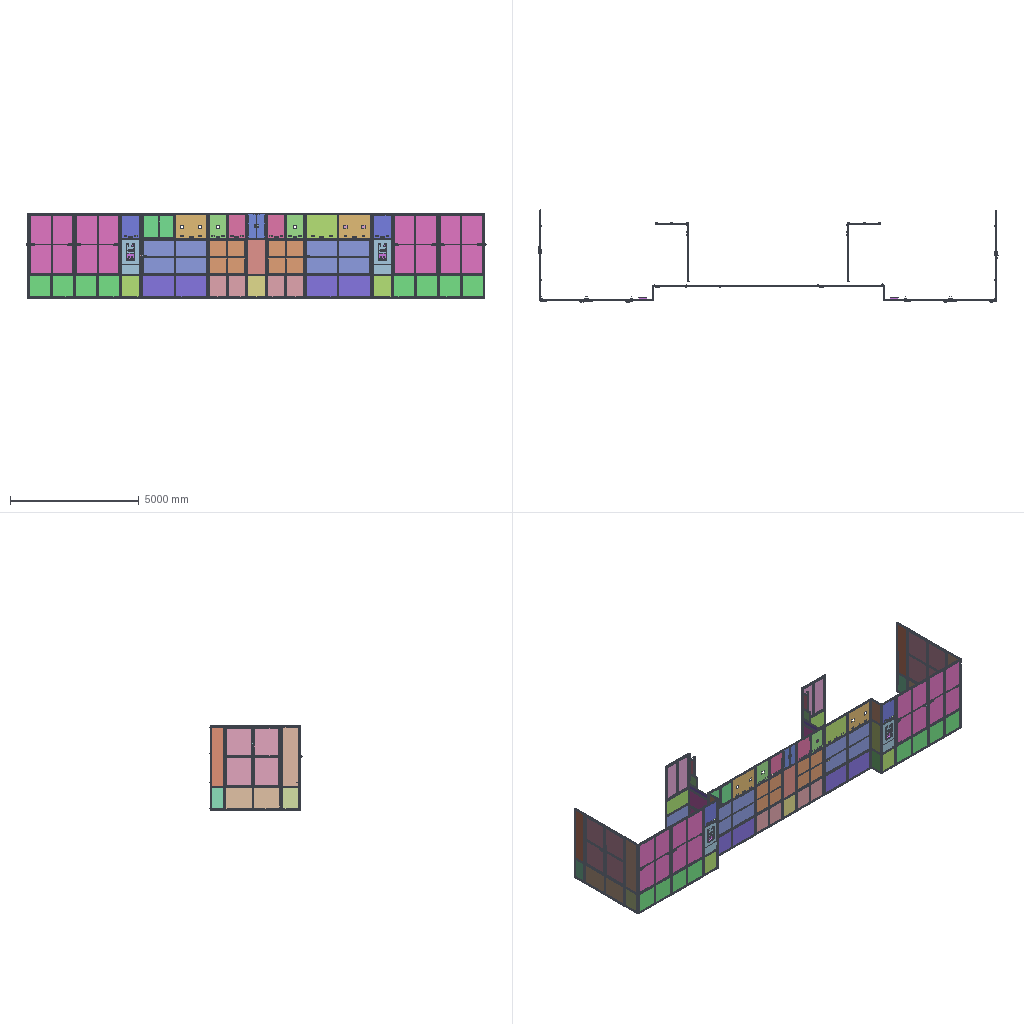Assembly | SolidWorks | 258 different items | 3509 placed | box 17871 x 3575 x 3280 mm
Parts list (item | name | quantity | parent item | size | volume | features):
1 | (subassembly) | x2 | in 6, 44 | - | 15381691 mm3 | features ReferencePattern 29, LocalLPattern 9
2 | (subassembly) | x2 | in 6, 44 | 1336 x 15 x 720 mm | 5449315 mm3 | features ReferencePattern 3, LocalLPattern 2
3 | (subassembly) | x2 | in 6, 44 | 1336 x 15 x 720 mm | 5449313 mm3 | features ReferencePattern 3, LocalLPattern 2
4 | (subassembly) | x2 | in 6, 44 | 685 x 936.5 x 44 mm | 1299683 mm3 | -
5 | (subassembly) | x2 | in 6, 44 | 685 x 936.5 x 44 mm | 1322747 mm3 | -
6 | (subassembly) | x1 | - | - | 28902679 mm3 | -
7 | (subassembly) | x1 | - | - | 60412715 mm3 | -
8 | (subassembly) | x1 | in 7 | - | 23168671 mm3 | features ReferencePattern 57, LocalLPattern 9, CompositeCurve 4, DerivedHolePattern 2
9 | (subassembly) | x1 | in 7 | 1225 x 936.5 x 44 mm | 2159359 mm3 | -
10 | (subassembly) | x1 | - | - | 65477431 mm3 | -
11 | (subassembly) | x1 | - | - | 15444382 mm3 | -
12 | (subassembly) | x1 | in 10 | - | 24079558 mm3 | features ReferencePattern 37, LocalLPattern 9, CompositeCurve 6
13 | (subassembly) | x2 | in 7, 10 | 1336 x 15 x 1260 mm | 9289979 mm3 | features ReferencePattern 3, LocalLPattern 2
14 | (subassembly) | x2 | in 7, 10 | 1336 x 89 x 1260 mm | 9587971 mm3 | features ReferencePattern 3, LocalLPattern 2
15 | (subassembly) | x2 | in 7, 10 | 595.4 x 40 x 3280 mm | 13933282 mm3 | features ReferencePattern 20, LocalLPattern 6
16 | (subassembly) | x1 | in 10 | 902 x 84 x 625 mm | 3238320 mm3 | features ReferencePattern 5, LocalLPattern 1
17 | (subassembly) | x1 | in 10 | 902 x 68 x 625 mm | 3235743 mm3 | features ReferencePattern 5, LocalLPattern 1
18 | (subassembly) | x2 | in 7, 10 | 1225 x 936.5 x 44 mm | 2112957 mm3 | -
19 | (subassembly) | x2 | - | 720.4 x 40 x 3280 mm | 15751167 mm3 | features ReferencePattern 12, LocalLPattern 4
20 | (subassembly) | x2 | - | - | - | -
21 | (subassembly) | x2 | in 20 | - | 17892849 mm3 | features ReferencePattern 36, LocalLPattern 3, DerivedHolePattern 1, MirrorCompFeat 1
22 | (subassembly) | x1 | in 11 | 772.4 x 40 x 3280 mm | 13403212 mm3 | features ReferencePattern 21, LocalLPattern 5, CompositeCurve 2
23 | (subassembly) | x4 | in 20 | - | - | features ReferencePattern 51, LocalLPattern 7, CompositeCurve 4
24 | (subassembly) | x2 | - | 562.4 x 40 x 3280 mm | 12898463 mm3 | features ReferencePattern 12, LocalLPattern 4
25 | (subassembly) | x2 | - | - | 29193097 mm3 | features ReferencePattern 104, MirrorCompFeat 10, LocalLPattern 4, DerivedHolePattern 1
26 | (subassembly) | x2 | - | - | 29490939 mm3 | -
27 | (subassembly) | x2 | in 26 | 40 x 3280 x 1290 mm | 16940253 mm3 | features ReferencePattern 22, LocalLPattern 5, MirrorCompFeat 2, CompositeCurve 1
28 | (subassembly) | x4 | in 26 | 633 x 92.5 x 1575 mm | 6275343 mm3 | features ReferencePattern 36, LocalLPattern 7, CompositeCurve 3
29 | (subassembly) | x4 | - | - | - | features CompositeCurve 1
30 | (subassembly) | x4 | in 29 | - | 16081270 mm3 | features ReferencePattern 57, LocalLPattern 5, CompositeCurve 3
31 | (subassembly) | x4 | in 29 | 2296 x 92.007 x 864.302 mm | 10874128 mm3 | features ReferencePattern 7, LocalLPattern 2
32 | (subassembly) | x4 | in 29 | - | 11302855 mm3 | features ReferencePattern 6, LocalLPattern 3
33 | (subassembly) | x2 | in 11 | 349.5 x 954 x 47.25 mm | 1020587 mm3 | features ReferencePattern 5, LocalLPattern 1
34 | (subassembly) | x526 | in 1, 8, 12, 15, 19, 21, 22, 23, 24, 25, 27, 28, 30, 41 | - | - | -
35 | (subassembly) | x4 | in 33 | 44.75 x 12.6 x 82 mm | 29571 mm3 | -
36 | (subassembly) | x2 | in 21 | - | - | -
37 | (subassembly) | x20 | in 23, 28 | 62 x 12.05 x 82 mm | 23876 mm3 | -
38 | (subassembly) | x16 | in 1, 8, 12, 30 | - | - | -
39 | (subassembly) | x1 | in 7 | - | 117384 mm3 | -
40 | (subassembly) | x2 | - | - | 12397020 mm3 | -
41 | (subassembly) | x2 | in 40 | 792.4 x 40 x 3280 mm | 8824321 mm3 | features ReferencePattern 12, LocalLPattern 3
42 | (subassembly) | x2 | in 40 | 697 x 1379 x 104.25 mm | 2244190 mm3 | features ReferencePattern 6, DerivedHolePattern 1
43 | (subassembly) | x2 | in 40 | 695 x 928.5 x 44 mm | 1328508 mm3 | -
44 | (subassembly) | x1 | - | - | 28902679 mm3 | -
45 | - | x2 | in 18 | 1225 x 925 x 38 mm | 1989320 mm3 | features ICE 7, SMWeldBead 4, EdgeFlange 2, FlatPattern 1, HoleWzd 1, SMBaseFlange 1, SheetMetal 1
46 | - | x8 | in 19, 24 | 14 x 20.3 x 2314 mm | 117819 mm3 | features BaseBody 1, ICE 1, MoveFace 1
47 | - | x4 | in 25 | 14 x 20.3 x 320 mm | 16293 mm3 | features BaseBody 1, ICE 1, MoveFace 1
48 | - | x4 | in 25 | 14 x 20.3 x 420 mm | 21385 mm3 | features BaseBody 1, ICE 1, MoveFace 1
49 | - | x20 | in 15, 24 | 14 x 20.3 x 410 mm | 20875 mm3 | features BaseBody 1, ICE 1, MoveFace 1
50 | - | x8 | in 28 | 14 x 20.3 x 461 mm | 23472 mm3 | features BaseBody 1, ICE 1, MoveFace 1
51 | - | x8 | in 19 | 14 x 20.3 x 568 mm | 28920 mm3 | features BaseBody 1, ICE 1, MoveFace 1
52 | - | x4 | in 41 | 14 x 20.3 x 606 mm | 30855 mm3 | features BaseBody 1, ICE 1, MoveFace 1
53 | - | x4 | in 22 | 14 x 20.3 x 620 mm | 31568 mm3 | features BaseBody 1, ICE 1, MoveFace 1
54 | - | x8 | in 1 | 14 x 20.3 x 657 mm | 33452 mm3 | features BaseBody 1, ICE 1, MoveFace 1
55 | - | x16 | in 25 | 14 x 20.3 x 670 mm | 34114 mm3 | features BaseBody 1, ICE 1, MoveFace 1
56 | - | x4 | in 32 | 23 x 25 x 60 mm | 5085 mm3 | features HoleWzd 2, Chamfer 1, FlatPattern 1, SMBaseFlange 1, SheetMetal 1
57 | - | x4 | in 27 | 14 x 20.3 x 692 mm | 35234 mm3 | features BaseBody 1, ICE 1, MoveFace 1
58 | - | x4 | in 25 | 14 x 20.3 x 730 mm | 37168 mm3 | features BaseBody 1, ICE 1, MoveFace 1
59 | - | x20 | in 1, 8, 12, 21, 30 | 14 x 20.3 x 786 mm | 40020 mm3 | features BaseBody 1, ICE 1, MoveFace 1
60 | - | x20 | in 21, 30 | 14 x 20.3 x 800 mm | 40733 mm3 | features BaseBody 1, ICE 1, MoveFace 1
61 | - | x4 | in 27 | 14 x 20.3 x 842 mm | 42871 mm3 | features BaseBody 1, ICE 1, MoveFace 1
62 | - | x37 | in 1, 8, 12, 15, 19, 22, 24, 30, 41 | 14 x 20.3 x 856 mm | 43584 mm3 | features BaseBody 1, ICE 1, MoveFace 1
63 | - | x4 | in 15 | 14 x 20.3 x 914 mm | 46537 mm3 | features BaseBody 1, ICE 1, MoveFace 1
64 | - | x16 | in 23 | 14 x 20.3 x 915 mm | 46588 mm3 | features BaseBody 1, ICE 1, MoveFace 1
65 | - | x8 | in 13, 14 | 30 x 15 x 1200 mm | 289403 mm3 | features BaseBody 1, MoveFace 1
66 | - | x4 | in 13, 14 | 30 x 15 x 1200 mm | 289001 mm3 | features BaseBody 1, HoleWzd 1, MoveFace 1
67 | - | x10 | in 16, 31 | 39 x 17 x 40 mm | 4045 mm3 | features HoleWzd 2, FlatPattern 1, SMBaseFlange 1, SheetMetal 1
68 | - | x4 | in 13, 14 | 30 x 15 x 1276 mm | 306850 mm3 | features HoleWzd 3, BaseBody 1, MoveFace 1
69 | - | x12 | in 2, 3, 13, 14 | 30 x 15 x 1276 mm | 307460 mm3 | features BaseBody 1, HoleWzd 1, MoveFace 1
70 | - | x8 | in 31, 32 | 30 x 15 x 2236 mm | 538276 mm3 | features HoleWzd 3, BaseBody 1, MoveFace 1
71 | - | x8 | in 31, 32 | 30 x 15 x 2236 mm | 538982 mm3 | features BaseBody 1, HoleWzd 1, MoveFace 1
72 | - | x4 | in 16, 17 | 30 x 15 x 565 mm | 136260 mm3 | features BaseBody 1, MoveFace 1
73 | - | x8 | in 2, 3 | 30 x 15 x 660 mm | 159171 mm3 | features BaseBody 1, MoveFace 1
74 | - | x4 | in 2, 3 | 30 x 15 x 660 mm | 158770 mm3 | features BaseBody 1, HoleWzd 1, MoveFace 1
75 | - | x20 | in 31, 32 | 30 x 15 x 802 mm | 193417 mm3 | features BaseBody 1, MoveFace 1
76 | - | x4 | in 32 | 30 x 15 x 802 mm | 193016 mm3 | features BaseBody 1, HoleWzd 1, MoveFace 1
77 | - | x2 | in 16, 17 | 30 x 15 x 842 mm | 202454 mm3 | features HoleWzd 2, BaseBody 1, MoveFace 1
78 | - | x18 | in 8, 30 | 17.5 x 17 x 60 mm | 3562 mm3 | features HoleWzd 2, FlatPattern 1, SMBaseFlange 1, SheetMetal 1
79 | - | x2 | in 16, 17 | 30 x 15 x 842 mm | 203064 mm3 | features BaseBody 1, MoveFace 1
80 | - | x2 | in 25 | 40 x 40 x 1548 mm | 930498 mm3 | features Extrusion 1
81 | - | x8 | in 25 | 40 x 40 x 2144 mm | 1280370 mm3 | features Extrusion 1, HoleWzd 1
82 | - | x2 | in 25 | 40 x 40 x 240 mm | 135882 mm3 | features Extrusion 1, HoleWzd 1
83 | - | x2 | in 25 | 40 x 40 x 2470 mm | 1483507 mm3 | features HoleWzd 2, Extrusion 1
84 | - | x4 | in 25 | 40 x 40 x 400 mm | 232057 mm3 | features Extrusion 1, HoleWzd 1
85 | - | x2 | in 25 | 40 x 40 x 410 mm | 238068 mm3 | features Extrusion 1, HoleWzd 1
86 | - | x2 | in 25 | 40 x 40 x 454 mm | 264516 mm3 | features Extrusion 1, HoleWzd 1
87 | - | x4 | in 25 | 40 x 40 x 730 mm | 430419 mm3 | features Extrusion 1, HoleWzd 1
88 | - | x4 | in 25 | 40 x 40 x 810 mm | 486492 mm3 | features HoleWzd 2, Extrusion 1
89 | - | x10 | in 17, 32 | 23 x 17 x 40 mm | 2765 mm3 | features HoleWzd 2, FlatPattern 1, SMBaseFlange 1, SheetMetal 1
90 | - | x2 | in 25 | 40 x 40 x 922 mm | 554211 mm3 | features Extrusion 1
91 | - | x8 | in 27 | 40 x 40 x 1210 mm | 708024 mm3 | features BaseBody 1, HoleWzd 1, MoveFace 1
92 | - | x8 | in 1 | 40 x 40 x 1420 mm | 832360 mm3 | features BaseBody 1, HoleWzd 1, MoveFace 1
93 | - | x12 | in 30 | 40 x 40 x 1705 mm | 1001101 mm3 | features BaseBody 1, HoleWzd 1, MoveFace 1
94 | - | x6 | in 21 | 40 x 40 x 2120 mm | 1246811 mm3 | features BaseBody 1, HoleWzd 1, MoveFace 1
95 | - | x8 | in 8, 12 | 40 x 40 x 2500 mm | 1471799 mm3 | features BaseBody 1, HoleWzd 1, MoveFace 1
96 | - | x3 | in 1, 12 | 40 x 40 x 3280 mm | 1938828 mm3 | features HoleWzd 5, BaseBody 1, MoveFace 1
97 | - | x3 | in 1, 12 | 40 x 40 x 3280 mm | 1938828 mm3 | features HoleWzd 5, BaseBody 1, MoveFace 1
98 | - | x4 | in 21 | 40 x 40 x 3280 mm | 1937764 mm3 | features HoleWzd 4, BaseBody 1, MoveFace 1
99 | - | x8 | in 19, 24 | 40 x 40 x 3280 mm | 1939169 mm3 | features HoleWzd 4, 3DProfileFeature 1, BaseBody 1, MoveFace 1
100 | - | x12 | in 21 | 72 x 17 x 32 mm | 6272 mm3 | features Chamfer 1, FlatPattern 1, HoleWzd 1, SMBaseFlange 1, SheetMetal 1
101 | - | x4 | in 27 | 40 x 40 x 3280 mm | 1937764 mm3 | features HoleWzd 4, BaseBody 1, MoveFace 1
102 | - | x16 | in 8, 15, 22, 30, 41 | 40 x 40 x 3280 mm | 1939654 mm3 | features HoleWzd 3, BaseBody 1, MoveFace 1
103 | - | x4 | in 30 | 40 x 40 x 3280 mm | 1938824 mm3 | features HoleWzd 5, BaseBody 1, MoveFace 1
104 | - | x6 | in 24 | 40 x 40 x 470 mm | 269890 mm3 | features BaseBody 1, HoleWzd 1, MoveFace 1
105 | - | x8 | in 15 | 40 x 40 x 503 mm | 289428 mm3 | features BaseBody 1, HoleWzd 1, MoveFace 1
106 | - | x6 | in 19 | 40 x 40 x 628 mm | 363437 mm3 | features BaseBody 1, HoleWzd 1, MoveFace 1
107 | - | x3 | in 22 | 40 x 40 x 680 mm | 394225 mm3 | features BaseBody 1, HoleWzd 1, MoveFace 1
108 | - | x8 | in 41 | 40 x 40 x 700 mm | 406067 mm3 | features BaseBody 1, HoleWzd 1, MoveFace 1
109 | - | x10 | in 1, 8, 12, 21, 30 | 40 x 40 x 846 mm | 492509 mm3 | features BaseBody 1, HoleWzd 1, MoveFace 1
110 | - | x4 | in 1, 8, 12 | 40 x 40 x 920 mm | 536323 mm3 | features BaseBody 1, HoleWzd 1, MoveFace 1
111 | - | x2 | in 21 | 43 x 52 x 100 mm | 25907 mm3 | features HoleWzd 2, FlatPattern 1, SMBaseFlange 1, SheetMetal 1
112 | - | x8 | in 28 | 40 x 40 x 1575 mm | 681555 mm3 | features BaseBody 1, MoveFace 1
113 | - | x8 | in 23 | 40 x 40 x 2310 mm | 999614 mm3 | features BaseBody 1, MoveFace 1
114 | - | x8 | in 28 | 40 x 40 x 521 mm | 219782 mm3 | features BaseBody 1, HoleWzd 1, MoveFace 1
115 | - | x12 | in 23 | 40 x 40 x 975 mm | 416243 mm3 | features BaseBody 1, HoleWzd 1, MoveFace 1
116 | - | x144 | in 2, 3, 13, 14, 16, 17, 31, 32 | 10.5 x 10.5 x 19.3 mm | 617.652 mm3 | features BaseBody 1
117 | - | x44 | in 8, 30, 32 | 7 x 7 x 0.5 mm | 15.221 mm3 | features Revolution 1
118 | - | x68 | in 1, 8, 12, 16, 17, 22, 31, 32 | 9 x 9 x 0.8 mm | 39.276 mm3 | features Revolution 1
119 | - | x68 | in 1, 8, 21, 30 | 10 x 10 x 1 mm | 56.478 mm3 | features Revolution 1
120 | - | x9 | in 4, 5, 9, 18, 43 | 115 x 31.4 x 143 mm | 78336 mm3 | features BaseBody 1
121 | - | x4 | in 21 | 9.187 x 9.2 x 1.2 mm | 53.532 mm3 | features Extrusion 1
122 | - | x4 | in 31 | 72 x 30 x 40 mm | 6134 mm3 | features HoleWzd 2, Chamfer 1, EdgeFlange 1, FlatPattern 1, SMBaseFlange 1, SheetMetal 1
123 | - | x6 | in 25 | 50 x 50 x 30 mm | 23521 mm3 | features BaseBody 1
124 | - | x4 | in 28 | 107 x 38 x 20.5 mm | 23344 mm3 | features BaseBody 1
125 | - | x1 | in 39 | - | - | features BaseBody 30, RefSurface 1
126 | - | x1 | in 39 | 35.586 x 51.386 x 50.3 mm | 17360 mm3 | features BaseBody 15
127 | - | x8 | in 25 | 1048 x 726 x 4 mm | 3043392 mm3 | features Extrusion 1
128 | - | x2 | in 25 | 2140 x 200 x 4 mm | 1712000 mm3 | features Extrusion 1, WeldmentFeature 1
129 | - | x2 | in 25 | 356 x 450 x 4 mm | 640800 mm3 | features Extrusion 1
130 | - | x2 | in 25 | 726 x 236 x 4 mm | 685344 mm3 | features Extrusion 1
131 | - | x4 | in 21 | 1037 x 843 x 5 mm | 4370955 mm3 | features Extrusion 1, HoleWzd 1
132 | - | x8 | in 23 | 972 x 1092 x 5 mm | 5307120 mm3 | features Extrusion 1, HoleWzd 1
133 | - | x8 | in 30 | 50 x 35 x 40 mm | 5650 mm3 | features HoleWzd 2, Chamfer 1, EdgeFlange 1, FlatPattern 1, SMBaseFlange 1, SheetMetal 1
134 | - | x16 | in 31, 32 | 818 x 1119 x 5 mm | 4576710 mm3 | features Extrusion 1
135 | - | x2 | in 27 | 1206 x 690 x 5 mm | 4160700 mm3 | features Extrusion 1, HoleWzd 1
136 | - | x2 | in 27 | 1206 x 842 x 5 mm | 5077260 mm3 | features Extrusion 1, HoleWzd 1
137 | - | x4 | in 8, 12 | 1226 x 842 x 5 mm | 5161460 mm3 | features Extrusion 1, HoleWzd 1
138 | - | x1 | in 22 | 1350 x 676 x 5 mm | 4563000 mm3 | features Extrusion 1, HoleWzd 1
139 | - | x4 | in 28 | 517 x 1491 x 5 mm | 3854235 mm3 | features Extrusion 1, HoleWzd 1
140 | - | x2 | in 24 | 466 x 2310 x 5 mm | 5382300 mm3 | features Extrusion 1, HoleWzd 1
141 | - | x2 | in 24 | 466 x 842 x 5 mm | 1961860 mm3 | features Extrusion 1, HoleWzd 1
142 | - | x2 | in 15 | 499 x 1350 x 5 mm | 3368250 mm3 | features Extrusion 1, HoleWzd 1
143 | - | x2 | in 15 | 499 x 842 x 5 mm | 2100790 mm3 | features Extrusion 1, HoleWzd 1
144 | - | x8 | in 23, 29 | 160 x 64 x 4 mm | 39767 mm3 | features HoleWzd 2, Extrusion 1, Fillet 1
145 | - | x2 | in 15 | 499 x 916 x 5 mm | 2285420 mm3 | features Extrusion 1, HoleWzd 1
146 | - | x2 | in 19 | 624 x 2310 x 5 mm | 7207200 mm3 | features Extrusion 1, HoleWzd 1
147 | - | x2 | in 19 | 624 x 842 x 5 mm | 2627040 mm3 | features Extrusion 1, HoleWzd 1
148 | - | x8 | in 2, 3 | 676 x 639 x 5 mm | 2159820 mm3 | features Extrusion 1
149 | - | x1 | in 22 | 676 x 842 x 5 mm | 2845960 mm3 | features Extrusion 1, HoleWzd 1
150 | - | x4 | in 1 | 686 x 842 x 5 mm | 2888060 mm3 | features Extrusion 1, HoleWzd 1
151 | - | x2 | in 41 | 696 x 842 x 5 mm | 2930160 mm3 | features Extrusion 1, HoleWzd 1
152 | - | x8 | in 30 | 829 x 842 x 5 mm | 3490090 mm3 | features Extrusion 1, HoleWzd 1
153 | - | x2 | in 16, 17 | 18 x 135 x 30 mm | 20354 mm3 | features BaseBody 1
154 | - | x4 | in 21 | 8 x 8 x 12 mm | 187.399 mm3 | features BaseBody 1, MoveFace 1
155 | - | x1 | in 12 | - | - | features BaseBody 9, RefSurface 6
156 | - | x4 | in 32 | 160 x 64 x 19 mm | 189875 mm3 | features HoleWzd 2, Extrusion 1, Fillet 1
157 | - | x20 | in 16, 17, 31, 32 | 8 x 8 x 20 mm | 286.49 mm3 | features BaseBody 1
158 | - | x16 | in 8, 12, 22 | 8 x 8 x 8 mm | 137.134 mm3 | features BaseBody 1, MoveFace 1
159 | - | x16 | in 33 | 10 x 10 x 12 mm | 284.359 mm3 | features BaseBody 1
160 | - | x36 | in 2, 3, 13, 14, 16, 17, 31, 32 | 32 x 32 x 15 mm | 8367 mm3 | features BaseBody 1
161 | - | x16 | in 23, 28 | 55 x 14.5 x 18 mm | 8175 mm3 | features BaseBody 1
162 | - | x18 | in 8, 30 | 17 x 15 x 50 mm | 8082 mm3 | features BaseBody 1
163 | - | x32 | in 25 | 10 x 6 x 6 mm | 253.469 mm3 | features BaseBody 1
164 | - | x8 | in 13, 14 | 1216 x 639 x 5 mm | 3885120 mm3 | features Extrusion 1
165 | - | x2 | in 16, 17 | 581 x 858 x 5 mm | 2492490 mm3 | features Extrusion 1
166 | - | x20 | in 4, 5, 9, 18, 33, 43 | 43 x 107 x 16 mm | 22651 mm3 | features BaseBody 1, ICE 1
167 | - | x8 | in 23 | 40 x 40 x 4 mm | 5920 mm3 | features HoleWzd 3, Extrusion 1, Fillet 1
168 | - | x8 | in 8, 12, 22 | 53 x 14 x 24.5 mm | 11695 mm3 | features BaseBody 1
169 | - | x2 | in 12 | 33.5 x 13.5 x 1230 mm | 229950 mm3 | features BaseBody 1, HoleWzd 1, ICE 1, MoveFace 1
170 | - | x4 | in 1 | 33.5 x 13.5 x 1420 mm | 265656 mm3 | features BaseBody 1, HoleWzd 1, ICE 1, MoveFace 1
171 | - | x8 | in 30 | 33.5 x 13.5 x 1705 mm | 319217 mm3 | features BaseBody 1, HoleWzd 1, ICE 1, MoveFace 1
172 | - | x4 | in 8, 12 | 33.5 x 13.5 x 2500 mm | 468220 mm3 | features ICE 2, BaseBody 1, HoleWzd 1, MoveFace 1
173 | - | x36 | in 2, 3, 13, 14, 16, 17, 31, 32 | 32 x 32 x 15 mm | 8036 mm3 | features BaseBody 1
174 | - | x4 | in 32 | 56 x 30 x 40 mm | 5174 mm3 | features HoleWzd 2, Chamfer 1, EdgeFlange 1, FlatPattern 1, SMBaseFlange 1, SheetMetal 1
175 | - | x1 | in 39 | 45 x 26 x 108 mm | 14308 mm3 | features HoleWzd 2, Fillet 1, FlatPattern 1, SMBaseFlange 1, SheetMetal 1
176 | - | x1 | in 39 | 68 x 17 x 50 mm | 7802 mm3 | features HoleWzd 2, Fillet 1, FlatPattern 1, SMBaseFlange 1, SheetMetal 1
177 | - | x8 | in 31, 32 | 16.002 x 50.042 x 18.313 mm | 6537 mm3 | features BaseBody 8
178 | - | x8 | in 30 | 16.008 x 126.481 x 28.318 mm | 9351 mm3 | features BaseBody 7
179 | - | x12 | in 23, 29, 32 | - | 237710 mm3 | features BaseBody 17, ICE 1
180 | - | x12 | in 23, 29, 30 | - | 135185 mm3 | features BaseBody 17
181 | - | x2 | in 33 | 330 x 954 x 38 mm | 933994 mm3 | features ICE 5, SMWeldBead 4, Chamfer 2, EdgeFlange 2, HoleWzd 2, FlatPattern 1, SMBaseFlange 1, SheetMetal 1
182 | - | x32 | in 1, 8, 12, 15, 22 | 13.8 x 7.5 x 8 mm | 622.996 mm3 | features BaseBody 1
183 | - | x132 | in 1, 8, 21, 23, 28, 30 | 19.5 x 6 x 8 mm | 667.11 mm3 | features BaseBody 1
184 | - | x84 | in 1, 8, 12, 21, 23, 28, 30, 33 | 19.5 x 6 x 8 mm | 631.457 mm3 | features BaseBody 1
185 | - | x144 | in 1, 8, 12, 15, 19, 21, 22, 23, 24, 28, 30, 41, 42 | 13.001 x 8.797 x 21 mm | 1304 mm3 | features BaseBody 1
186 | - | x4 | in 21 | 11.5 x 6.2 x 17 mm | 1002 mm3 | features BaseBody 1
187 | - | x20 | in 37 | 36.75 x 12.05 x 79 mm | 10360 mm3 | features BaseBody 1
188 | - | x20 | in 37 | 7 x 7 x 82 mm | 3156 mm3 | features BaseBody 1
189 | - | x20 | in 37 | 36.75 x 12.05 x 79 mm | 10360 mm3 | features BaseBody 1
190 | - | x4 | in 35 | 44.75 x 12.05 x 79 mm | 13207 mm3 | features BaseBody 1
191 | - | x4 | in 35 | 7 x 7 x 82 mm | 3156 mm3 | features BaseBody 1
192 | - | x2 | in 42 | 697 x 1351 x 38 mm | 1680620 mm3 | features SMWeldBead 4, HoleWzd 3, EdgeFlange 2, BossThin 1, FlatPattern 1, ICE 1, SMBaseFlange 1, SheetMetal 1
193 | - | x4 | in 35 | 44.75 x 12.05 x 79 mm | 13207 mm3 | features BaseBody 1
194 | - | x8 | in 25 | 9.5 x 13.5 x 140 mm | 13278 mm3 | features BaseBody 1
195 | - | x8 | in 42 | 8 x 9.238 x 2.7 mm | 105.377 mm3 | features BaseBody 1
196 | - | x56 | in 8, 30 | 5.5 x 6.351 x 2.4 mm | 50.752 mm3 | features BaseBody 1
197 | - | x36 | in 8, 30 | 7 x 8.083 x 3.2 mm | 107.56 mm3 | features BaseBody 1
198 | - | x4 | in 21 | 8 x 9.238 x 4 mm | 165.049 mm3 | features BaseBody 1
199 | - | x36 | in 8, 30 | 5.5 x 5.5 x 11 mm | 117.558 mm3 | features ICE 2, Chamfer 1, RevCut 1, Revolution 1
200 | - | x58 | in 16, 17, 31, 32, 39 | 7 x 7 x 12 mm | 234.462 mm3 | features ICE 3, Chamfer 1, RevCut 1, Revolution 1
201 | - | x120 | in 1, 8, 21, 23, 28, 30, 39 | 17 x 8.5 x 8.5 mm | 477.486 mm3 | features ICE 1, RevCut 1, Revolution 1
202 | - | x4 | in 21 | 8.5 x 8.5 x 21 mm | 554.737 mm3 | features ICE 2, Chamfer 1, RevCut 1, Revolution 1
203 | - | x2 | in 42 | 337 x 637 x 100 mm | 553796 mm3 | features EdgeFlange 5, ICE 2, Chamfer 1, FlatPattern 1, HoleWzd 1, SMBaseFlange 1, SheetMetal 1
204 | - | x8 | in 42 | 18 x 10 x 10 mm | 732.461 mm3 | features ICE 1, RevCut 1, Revolution 1
205 | - | x8 | in 28 | 10 x 10 x 24 mm | 898.677 mm3 | features Chamfer 2, ICE 2, RevCut 1, Revolution 1
206 | - | x16 | in 31, 32 | 10 x 10 x 36 mm | 1238 mm3 | features Chamfer 2, ICE 2, RevCut 1, Revolution 1
207 | - | x92 | in 1, 8, 12, 15, 19, 21, 22, 24, 25, 30, 41 | 10 x 10 x 46 mm | 1521 mm3 | features Chamfer 2, ICE 2, RevCut 1, Revolution 1
208 | - | x20 | in 1, 8, 12, 22 | 7.6 x 7.6 x 14.2 mm | 222.779 mm3 | features BaseBody 1
209 | - | x8 | in 42 | 9.5 x 9.5 x 10.75 mm | 302.249 mm3 | features BaseBody 1
210 | - | x36 | in 8, 30 | 8 x 8 x 10 mm | 162.002 mm3 | features BaseBody 1
211 | - | x60 | in 23, 28 | 12 x 12 x 15 mm | 531.654 mm3 | features BaseBody 1
212 | - | x60 | in 23, 28 | 12 x 12 x 25 mm | 814.397 mm3 | features BaseBody 1
213 | - | x66 | in 1, 8, 12, 23, 30 | 12 x 12 x 12 mm | 460.573 mm3 | features Chamfer 1, ICE 1, Revolution 1
214 | - | x2 | in 43 | 695 x 917 x 38 mm | 1204871 mm3 | features ICE 6, SMWeldBead 4, EdgeFlange 2, FlatPattern 1, SMBaseFlange 1, SheetMetal 1
215 | - | x8 | in 21 | 10 x 10 x 31 mm | 1100 mm3 | features BaseBody 1
216 | - | x6 | in 25 | 42 x 42 x 35 mm | 15839 mm3 | features BaseBody 1
217 | - | x8 | in 21 | 10.8 x 17.5 x 1010 mm | 79589 mm3 | features BaseBody 1, MoveFace 1
218 | - | x16 | in 25 | 10.8 x 17.5 x 1020 mm | 80377 mm3 | features BaseBody 1, MoveFace 1
219 | - | x16 | in 23 | 10.8 x 17.5 x 1090 mm | 85893 mm3 | features BaseBody 1, MoveFace 1
220 | - | x8 | in 27 | 10.8 x 17.5 x 1150 mm | 90621 mm3 | features BaseBody 1, MoveFace 1
221 | - | x8 | in 8, 12 | 10.8 x 17.5 x 1197 mm | 94324 mm3 | features BaseBody 1, MoveFace 1
222 | - | x6 | in 15, 22 | 10.8 x 17.5 x 1348 mm | 106223 mm3 | features BaseBody 1, MoveFace 1
223 | - | x8 | in 28 | 10.8 x 17.5 x 1495 mm | 117807 mm3 | features BaseBody 1, MoveFace 1
224 | - | x4 | in 25 | 10.8 x 17.5 x 180 mm | 14184 mm3 | features BaseBody 1, MoveFace 1
225 | - | x2 | in 4 | 685 x 925 x 38 mm | 1176046 mm3 | features ICE 7, SMWeldBead 4, EdgeFlange 2, FlatPattern 1, SMBaseFlange 1, SheetMetal 1
226 | - | x4 | in 25 | 10.8 x 17.5 x 199 mm | 15681 mm3 | features BaseBody 1, MoveFace 1
227 | - | x4 | in 25 | 10.8 x 17.5 x 2084 mm | 164220 mm3 | features BaseBody 1, MoveFace 1
228 | - | x8 | in 19, 24 | 10.8 x 17.5 x 1171 mm | 92275 mm3 | features BaseBody 1, MoveFace 1
229 | - | x4 | in 25 | 10.8 x 17.5 x 320 mm | 25216 mm3 | features BaseBody 1, MoveFace 1
230 | - | x4 | in 25 | 10.8 x 17.5 x 419 mm | 33017 mm3 | features BaseBody 1, MoveFace 1
231 | - | x20 | in 15, 24 | 10.8 x 17.5 x 410 mm | 32308 mm3 | features BaseBody 1, MoveFace 1
232 | - | x8 | in 28 | 10.8 x 17.5 x 461 mm | 36327 mm3 | features BaseBody 1, MoveFace 1
233 | - | x8 | in 19 | 10.8 x 17.5 x 568 mm | 44759 mm3 | features BaseBody 1, MoveFace 1
234 | - | x4 | in 41 | 10.8 x 17.5 x 606 mm | 47753 mm3 | features BaseBody 1, MoveFace 1
235 | - | x4 | in 22 | 10.8 x 17.5 x 620 mm | 48856 mm3 | features BaseBody 1, MoveFace 1
236 | - | x2 | in 5 | 685 x 925 x 38 mm | 1199110 mm3 | features ICE 6, SMWeldBead 4, EdgeFlange 2, FlatPattern 1, HoleWzd 1, SMBaseFlange 1, SheetMetal 1
237 | - | x8 | in 1 | 10.8 x 17.5 x 657 mm | 51772 mm3 | features BaseBody 1, MoveFace 1
238 | - | x16 | in 25 | 10.8 x 17.5 x 670 mm | 52796 mm3 | features BaseBody 1, MoveFace 1
239 | - | x4 | in 27 | 10.8 x 17.5 x 692 mm | 54530 mm3 | features BaseBody 1, MoveFace 1
240 | - | x4 | in 25 | 10.8 x 17.5 x 730 mm | 57524 mm3 | features BaseBody 1, MoveFace 1
241 | - | x20 | in 1, 8, 12, 21, 30 | 10.8 x 17.5 x 786 mm | 61937 mm3 | features BaseBody 1, MoveFace 1
242 | - | x20 | in 21, 30 | 10.8 x 17.5 x 800 mm | 63040 mm3 | features BaseBody 1, MoveFace 1
243 | - | x4 | in 27 | 10.8 x 17.5 x 842 mm | 66350 mm3 | features BaseBody 1, MoveFace 1
244 | - | x34 | in 1, 8, 12, 15, 19, 22, 24, 30, 41 | 10.8 x 17.5 x 856 mm | 67453 mm3 | features BaseBody 1, MoveFace 1
245 | - | x4 | in 15 | 10.8 x 17.5 x 914 mm | 72024 mm3 | features BaseBody 1, MoveFace 1
246 | - | x16 | in 23 | 10.8 x 17.5 x 915 mm | 72103 mm3 | features BaseBody 1, MoveFace 1
247 | - | x1 | in 9 | 1225 x 925 x 38 mm | 2035721 mm3 | features ICE 6, SMWeldBead 4, EdgeFlange 2, FlatPattern 1, HoleWzd 1, SMBaseFlange 1, SheetMetal 1
248 | - | x8 | in 21 | 14 x 20.3 x 1010 mm | 51425 mm3 | features BaseBody 1, ICE 1, MoveFace 1
249 | - | x16 | in 25 | 14 x 20.3 x 1020 mm | 51934 mm3 | features BaseBody 1, ICE 1, MoveFace 1
250 | - | x16 | in 23 | 14 x 20.3 x 1090 mm | 55498 mm3 | features BaseBody 1, ICE 1, MoveFace 1
251 | - | x8 | in 27 | 14 x 20.3 x 1150 mm | 58553 mm3 | features BaseBody 1, ICE 1, MoveFace 1
252 | - | x8 | in 8, 12 | 14 x 20.3 x 1197 mm | 60946 mm3 | features BaseBody 1, ICE 1, MoveFace 1
253 | - | x6 | in 15, 22 | 14 x 20.3 x 1348 mm | 68634 mm3 | features BaseBody 1, ICE 1, MoveFace 1
254 | - | x8 | in 28 | 14 x 20.3 x 1495 mm | 76119 mm3 | features BaseBody 1, ICE 1, MoveFace 1
255 | - | x4 | in 25 | 14 x 20.3 x 180 mm | 9165 mm3 | features BaseBody 1, ICE 1, MoveFace 1
256 | - | x4 | in 25 | 14 x 20.3 x 199 mm | 10132 mm3 | features BaseBody 1, ICE 1, MoveFace 1
257 | - | x4 | in 25 | 14 x 20.3 x 2084 mm | 106108 mm3 | features BaseBody 1, ICE 1, MoveFace 1
258 | - | x2 | in 14 | - | - | features BaseBody 14, RefSurface 6
Mates (type | each side: item.copy, entity, surface, feature), first 406 of 1867 lines:
In the top assembly
Coincident | 102.1 face plane 输入1 | 102.2 face plane 输入1 | 2 times
Coincident | 102.3 face plane 输入1 | 102.4 face plane 输入1 | 2 times
Coincident | 105.1 face plane 输入1 | 108.1 face plane 输入1
Coincident | 108.1 face plane 输入1 | 93.1 face plane 输入1
Coincident | 108.2 face plane 输入1 | 93.2 face plane 输入1
Coincident | 93.2 face plane 输入1 | 93.3 face plane 输入1
Coincident | 102.5 face plane 输入1 | 103.1 face plane 输入1 | 2 times
Coincident | 102.6 face plane 输入1 | 103.2 face plane 输入1 | 2 times
Coincident | 105.2 face plane 输入1 | 108.2 face plane 输入1
Coincident | 102.7 face plane 输入1 | 102.8 face plane 输入1 | 2 times
Coincident | 102.1 face plane 输入1 | 101.1 face plane 输入1
Coincident | 92.1 face plane 输入1 | 95.1 face plane 输入1
Coincident | 96.1 face plane 输入1 | 96.2 face plane 输入1 | 2 times
Coincident | 92.2 face plane 输入1 | 95.2 face plane 输入1
Coincident | 97.1 face plane 输入1 | 102.9 face plane 输入1 | 2 times
Coincident | 107.1 face plane 输入1 | 92.1 face plane 输入1
Coincident | 102.10 face plane 输入1 | 97.2 face plane 输入1 | 2 times
Coincident | 97.1 face plane 输入1 | 102.11 face plane 输入1
Coincident | 96.3 face plane 输入1 | 102.11 face plane 输入1
Coincident | 92.2 face plane 输入1 | 107.1 face plane 输入1
Coincident | 98.1 face plane 输入1 | 99.1 face plane 输入1 | 3 times
Coincident | 98.2 face plane 输入1 | 99.2 face plane 输入1 | 3 times
Coincident | 98.3 face plane 输入1 | 99.3 face plane 输入1 | 3 times
Coincident | 106.1 face plane 输入1 | 98.4 face plane 输入1
Coincident | 99.4 face plane 输入1 | 98.4 face plane 输入1
Coincident | 106.2 face plane 输入1 | 98.4 face plane 输入1
Coincident | 99.5 face plane 输入1 | 103.3 face plane 输入1 | 3 times
Coincident | 83.1 face plane Boss-Extrude 1 | 101.2 face plane 输入1 | 2 times
Coincident | 88.1 face plane Boss-Extrude 1 | 101.2 face plane 输入1
Coincident | 101.3 face plane 输入1 | 83.2 face plane Boss-Extrude 1 | 2 times
Coincident | 101.4 face plane 输入1 | 101.2 face plane 输入1
Coincident | 101.3 face plane 输入1 | 88.2 face plane Boss-Extrude 1
Coincident | 93.1 face plane 输入1 | 93.4 face plane 输入1
Coincident | 103.4 face plane 输入1 | 102.12 face plane 输入1 | 2 times
Coincident | 99.6 face plane 输入1 | 102.13 face plane 输入1 | 3 times
In subassembly 40
Coincident | 102.14 face plane 输入1 | 192.1 face plane Base-Flange 1
DistanceDim | 192.1 face plane Edge-Flange 1 | 102.14 face plane 输入1
DistanceDim | 192.1 face plane Edge-Flange 1 | 108.3 face plane 输入1
Coincident | 102.14 face plane 输入1 | 214.1 face plane Base-Flange 1
DistanceDim | 214.1 face plane Edge-Flange 1 | 102.14 face plane 输入1
DistanceDim | 214.1 face plane Edge-Flange 1 | 108.4 face plane 输入1
In subassembly 42
DistanceDim | 185.1 face plane 输入1 | 192.2 face plane Edge-Flange 1
Parallel | 192.2 face plane Edge-Flange 2 | 185.1 face plane 输入1
Concentric | 192.2 face cylinder M6 间隙Hole 1 | 185.1 face cylinder 输入1
Coincident | 185.1 face plane 输入1 | 185.2 face plane 输入1
Concentric | 192.2 face cylinder M6 间隙Hole 1 | 204.1 face cylinder Revolve 1
Coincident | 192.2 face plane Edge-Flange 1 | 204.1 face plane Revolve 1
Concentric | 192.2 face cylinder M6 间隙Hole 1 | 204.2 face cylinder Revolve 1
Coincident | 192.2 face plane Edge-Flange 1 | 204.2 face plane Revolve 1
Concentric | 192.2 face cylinder M6 间隙Hole 1 | 204.3 face cylinder Revolve 1
Coincident | 192.2 face plane Edge-Flange 1 | 204.3 face plane Revolve 1
Concentric | 192.2 face cylinder M6 间隙Hole 1 | 204.4 face cylinder Revolve 1
Coincident | 192.2 face plane Edge-Flange 1 | 204.4 face plane Revolve 1
DistanceDim | 185.3 face plane 输入1 | 192.2 face plane Edge-Flange 1
Concentric | 204.4 face cylinder Revolve 1 | 185.3 face cylinder 输入1
Coincident | 185.3 face plane 输入1 | 185.4 face plane 输入1
Concentric | 204.3 face cylinder Revolve 1 | 185.4 face cylinder 输入1
Coincident | 192.2 face plane Base-Flange 1 | 203.1 face plane Edge-Flange 7
Width | 203.1 face plane Edge-Flange 1 | 203.1 face plane Edge-Flange 1 | 192.2 face plane Cut-Extrude 1 | 192.2 face plane Cut-Extrude 1 | 2 times
Concentric | 192.2 face cylinder M5 间隙Hole 1 | 209.1 face cone 输入1
Coincident | 192.2 face plane Base-Flange 1 | 209.1 face plane 输入1
Concentric | 209.1 face cone 输入1 | 195.1 face cone 输入1
Coincident | 203.1 face plane Edge-Flange 5 | 195.1 face plane 输入1
In subassembly 41
Coincident | 102.15 face plane 输入1 | 108.5 face plane 输入1 | 3 times
Coincident | 108.5 face plane 输入1 | 102.16 face plane 输入1 | 3 times
Coincident | 108.6 face plane 输入1 | 102.16 face plane 输入1
Coincident | 102.15 face plane 输入1 | 108.7 face plane 输入1 | 2 times
Coincident | 102.15 face plane 输入1 | 108.6 face plane 输入1 | 2 times
Coincident | 108.7 face plane 输入1 | 234.1 face plane 输入1
Coincident | 108.7 face plane 输入1 | 234.1 edge
Coincident | 151.1 face plane Boss-Extrude 1 | 234.1 face plane 输入1
Coincident | 151.1 face plane Boss-Extrude 1 | 244.1 face plane 输入1
Coincident | 102.15 face plane 输入1 | 244.1 edge
Coincident | 151.1 face plane Boss-Extrude 1 | 234.2 face plane 输入1
Coincident | 108.5 face plane 输入1 | 234.2 edge
Coincident | 108.7 face plane 输入1 | 52.1 face plane 输入1
Coincident | 151.1 face plane Boss-Extrude 1 | 52.1 face plane 输入1 | 2 times
Coincident | 234.1 face plane 输入1 | 52.1 face plane 输入1
Coincident | 102.15 face plane 输入1 | 62.1 face plane 输入1
Coincident | 151.1 face plane Boss-Extrude 1 | 62.1 face plane 输入1 | 2 times
Width | 62.1 face plane 输入1 | 62.1 face plane 输入1 | 108.5 face plane 输入1 | 108.7 face plane 输入1
Coincident | 244.1 face plane 输入1 | 62.1 face plane 输入1
Coincident | 108.5 face plane 输入1 | 52.2 face plane 输入1
Coincident | 151.1 face plane Boss-Extrude 1 | 52.2 face plane 输入1
Coincident | 52.1 face plane 输入1 | 52.2 face plane 输入1
Coincident | 234.2 face plane 输入1 | 52.2 face plane 输入1
Coincident | 108.5 face plane 输入1 | 41.1 face | 4 times
Concentric | 108.5 face cylinder Ø19.0 (19) DiameterHole 1 | 41.1 face | 3 times
Concentric | 41.1 face | 41.1 face
Coincident | 244.1 face plane 输入1 | 244.2 face plane 输入1
Coincident | 102.16 face plane 输入1 | 244.2 edge
Coincident | 102.16 face plane 输入1 | 62.2 face plane 输入1
Coincident | 244.2 face plane 输入1 | 62.2 face plane 输入1
Coincident | 102.16 face plane 输入1 | 185.1 face plane 输入1
Concentric | 102.16 face cylinder M6 六角凹头Screw的柱形沉头Hole 1 | 185.1 face cylinder 输入1
Coincident | 185.1 face plane 输入1 | 185.2 face plane 输入1
Coincident | 185.2 face plane 输入1 | 185.5 face plane 输入1
Coincident | 185.5 face plane 输入1 | 185.6 face plane 输入1
Concentric | 102.16 face cylinder M6 六角凹头Screw的柱形沉头Hole 1 | 185.2 face cylinder 输入1
Concentric | 102.16 face cylinder M6 六角凹头Screw的柱形沉头Hole 1 | 185.5 face cylinder 输入1
Concentric | 102.16 face cylinder M6 六角凹头Screw的柱形沉头Hole 1 | 185.6 face cylinder 输入1
Concentric | 102.15 face cylinder M6 六角凹头Screw的柱形沉头Hole 1 | 207.1 face cylinder Revolve 1
Coincident | 102.15 face plane 输入1 | 207.1 face plane Revolve 1
Concentric | 102.15 face cylinder M6 六角凹头Screw的柱形沉头Hole 1 | 207.2 face cylinder Revolve 1
Coincident | 102.15 face plane 输入1 | 207.2 face plane Revolve 1
Concentric | 102.15 face cylinder M6 六角凹头Screw的柱形沉头Hole 1 | 207.3 face cylinder Revolve 1
Coincident | 102.15 face plane 输入1 | 207.3 face plane Revolve 1
Concentric | 102.15 face cylinder M6 六角凹头Screw的柱形沉头Hole 1 | 207.4 face cylinder Revolve 1
Coincident | 102.15 face plane 输入1 | 207.4 face plane Revolve 1
DistanceDim | 108.7 face plane 输入1 | 108.5 face plane 输入1
DistanceDim | 52.1 face plane 输入1 | 102.16 face plane 输入1
Coincident | 102.16 face plane 输入1 | 108.8 face plane 输入1 | 2 times
DistanceDim | 108.8 face plane 输入1 | 108.6 face plane 输入1
In subassembly 43
Width | 166.1 face plane 输入1 | 166.1 face plane 输入1 | 214.2 face plane Cut-Extrude 1 | 214.2 face plane Cut-Extrude 1
DistanceDim | 166.1 face plane 输入1 | 214.2 face plane Cut-Extrude 1
Coincident | 214.2 face plane Base-Flange 1 | 166.1 face plane 输入1
DistanceDim | 166.2 face plane 输入1 | 214.2 face plane Cut-Extrude 1 | 2 times
Coincident | 214.2 face plane Base-Flange 1 | 166.2 face plane 输入1
Coincident | 214.2 face plane Base-Flange 1 | 120.1 face plane 输入1
Concentric | 214.2 face cylinder Cut-Extrude 3 | 120.1 face cylinder 输入1 | 2 times
In subassembly 24
Coincident | 99.7 face plane 输入1 | 104.1 face plane 输入1 | 3 times
Coincident | 104.1 face plane 输入1 | 99.8 face plane 输入1 | 3 times
Coincident | 99.7 face plane 输入1 | 104.2 face plane 输入1 | 3 times
Coincident | 99.7 face plane 输入1 | 104.3 face plane 输入1 | 2 times
Coincident | 104.3 face plane 输入1 | 231.1 face plane 输入1
Coincident | 104.3 face plane 输入1 | 231.1 edge
Coincident | 141.1 face plane Boss-Extrude 1 | 231.1 face plane 输入1
Coincident | 141.1 face plane Boss-Extrude 1 | 244.1 face plane 输入1
Coincident | 99.7 face plane 输入1 | 244.1 edge
Coincident | 141.1 face plane Boss-Extrude 1 | 231.2 face plane 输入1
Coincident | 104.1 face plane 输入1 | 231.2 edge
Coincident | 104.3 face plane 输入1 | 49.1 face plane 输入1
Coincident | 141.1 face plane Boss-Extrude 1 | 49.1 face plane 输入1 | 2 times
Coincident | 231.1 face plane 输入1 | 49.1 face plane 输入1
Coincident | 99.7 face plane 输入1 | 62.1 face plane 输入1
Coincident | 141.1 face plane Boss-Extrude 1 | 62.1 face plane 输入1 | 2 times
Width | 62.1 face plane 输入1 | 62.1 face plane 输入1 | 104.1 face plane 输入1 | 104.3 face plane 输入1
Coincident | 244.1 face plane 输入1 | 62.1 face plane 输入1
Coincident | 104.1 face plane 输入1 | 49.2 face plane 输入1
Coincident | 141.1 face plane Boss-Extrude 1 | 49.2 face plane 输入1
Coincident | 49.1 face plane 输入1 | 49.2 face plane 输入1
Coincident | 231.2 face plane 输入1 | 49.2 face plane 输入1
Coincident | 104.1 face plane 输入1 | 24.1 face | 4 times
Concentric | 104.1 face cylinder Ø19.0 (19) DiameterHole 1 | 24.1 face | 3 times
Concentric | 24.1 face | 24.1 face
Coincident | 244.1 face plane 输入1 | 244.2 face plane 输入1
Coincident | 99.8 face plane 输入1 | 244.2 edge
Coincident | 99.8 face plane 输入1 | 62.2 face plane 输入1
Coincident | 244.2 face plane 输入1 | 62.2 face plane 输入1
Coincident | 99.8 face plane 输入1 | 185.1 face plane 输入1
Concentric | 99.8 face cylinder M6 六角凹头Screw的柱形沉头Hole 1 | 185.1 face cylinder 输入1
Coincident | 185.1 face plane 输入1 | 185.2 face plane 输入1
Coincident | 185.2 face plane 输入1 | 185.5 face plane 输入1
Coincident | 185.5 face plane 输入1 | 185.6 face plane 输入1
Concentric | 99.8 face cylinder M6 六角凹头Screw的柱形沉头Hole 1 | 185.2 face cylinder 输入1
Concentric | 99.8 face cylinder M6 六角凹头Screw的柱形沉头Hole 1 | 185.5 face cylinder 输入1
Concentric | 99.8 face cylinder M6 六角凹头Screw的柱形沉头Hole 1 | 185.6 face cylinder 输入1
Concentric | 99.7 face cylinder M6 六角凹头Screw的柱形沉头Hole 1 | 207.1 face cylinder Revolve 1
Coincident | 99.7 face plane 输入1 | 207.1 face plane Revolve 1
Concentric | 99.7 face cylinder M6 六角凹头Screw的柱形沉头Hole 1 | 207.2 face cylinder Revolve 1
Coincident | 99.7 face plane 输入1 | 207.2 face plane Revolve 1
Concentric | 99.7 face cylinder M6 六角凹头Screw的柱形沉头Hole 1 | 207.3 face cylinder Revolve 1
Coincident | 99.7 face plane 输入1 | 207.3 face plane Revolve 1
Concentric | 99.7 face cylinder M6 六角凹头Screw的柱形沉头Hole 1 | 207.4 face cylinder Revolve 1
Coincident | 99.7 face plane 输入1 | 207.4 face plane Revolve 1
DistanceDim | 104.3 face plane 输入1 | 104.1 face plane 输入1
DistanceDim | 49.1 face plane 输入1 | 99.8 face plane 输入1
Coincident | 141.1 face plane Boss-Extrude 1 | 140.1 face plane Boss-Extrude 1
Coincident | 140.1 face plane Boss-Extrude 1 | 46.1 face plane 输入1 | 2 times
Coincident | 99.8 face plane 输入1 | 46.1 face plane 输入1
Coincident | 141.1 face plane Boss-Extrude 1 | 62.2 face plane 输入1
DistanceDim | 46.1 face plane 输入1 | 104.3 face plane 输入1
Coincident | 49.3 face plane 输入1 | 140.1 face plane Boss-Extrude 1
Coincident | 140.1 face plane Boss-Extrude 1 | 228.1 face plane 输入1
Coincident | 228.1 face plane 输入1 | 46.1 face plane 输入1
Coincident | 99.8 face plane 输入1 | 228.1 edge
Coincident | 140.1 face plane Boss-Extrude 1 | 46.2 face plane 输入1
Coincident | 99.7 face plane 输入1 | 46.2 face plane 输入1
DistanceDim | 46.2 face plane 输入1 | 104.3 face plane 输入1
Coincident | 140.1 face plane Boss-Extrude 1 | 228.2 face plane 输入1
Coincident | 46.2 face plane 输入1 | 228.2 face plane 输入1
Coincident | 99.7 face plane 输入1 | 228.2 edge
In subassembly 10
DistanceDim | 69.1 face plane 输入1 | 95.3 face plane 输入1
DistanceDim | 160.1 face plane 输入1 | 95.4 face plane 输入1
DistanceDim | 68.1 face plane 输入1 | 95.3 face plane 输入1
DistanceDim | 160.2 face plane 输入1 | 95.4 face plane 输入1
LimitDistanceDim | 160.2 face plane 输入1 | 97.3 face plane 输入1
LimitDistanceDim | 96.4 face plane 输入1 | 160.3 face plane 输入1
Coincident | 96.4 face plane 输入1 | 45.1 face plane Base-Flange 1
DistanceDim | 45.1 face plane Edge-Flange 1 | 96.4 face plane 输入1
Coincident | 95.5 face plane 输入1 | 105.3 face plane 输入1
Coincident | 97.3 face plane 输入1 | 102.17 face plane 输入1 | 2 times
DistanceDim | 45.1 face plane Edge-Flange 1 | 95.4 face plane 输入1
DistanceDim | 79.1 face plane 输入1 | 110.1 face plane 输入1
DistanceDim | 173.1 face plane 输入1 | 95.4 face plane 输入1
DistanceDim | 77.1 face plane 输入1 | 95.6 face plane 输入1
DistanceDim | 173.2 face plane 输入1 | 95.4 face plane 输入1
Coincident | 97.3 face plane 输入1 | 173.2 face plane 输入1
Coincident | 110.1 face plane 输入1 | 173.3 face plane 输入1
In subassembly 16
Coincident | 72.1 face plane 输入1 | 160.4 face plane 输入1 | 3 times
Coincident | 72.1 face plane 输入1 | 160.5 face plane 输入1 | 3 times
Coincident | 160.4 face plane 输入1 | 77.2 face plane 输入1 | 3 times
Coincident | 72.1 face plane 输入1 | 79.2 face plane 输入1
Coincident | 160.5 face plane 输入1 | 79.2 face plane 输入1 | 2 times
Coincident | 77.2 face plane 输入1 | 72.2 face plane 输入1
Coincident | 77.2 face plane 输入1 | 173.4 face plane 输入1 | 3 times
Coincident | 173.4 face plane 输入1 | 72.2 face plane 输入1 | 2 times
Coincident | 79.2 face plane 输入1 | 173.5 face plane 输入1 | 2 times
Coincident | 173.5 face plane 输入1 | 72.2 face plane 输入1
Concentric | 160.5 face cylinder 输入1 | 116.1 face cylinder 输入1
Coincident | 160.5 face plane 输入1 | 116.1 face plane 输入1
Concentric | 160.5 face cylinder 输入1 | 116.2 face cylinder 输入1
Coincident | 160.5 face plane 输入1 | 116.2 face plane 输入1
Concentric | 160.4 face cylinder 输入1 | 116.3 face cylinder 输入1
Coincident | 160.4 face plane 输入1 | 116.3 face plane 输入1
Coincident | 160.4 face plane 输入1 | 116.4 face plane 输入1
Concentric | 160.4 face cylinder 输入1 | 116.4 face cylinder 输入1
Concentric | 173.4 face cylinder 输入1 | 116.5 face cylinder 输入1
Coincident | 173.4 face plane 输入1 | 116.5 face plane 输入1
Concentric | 173.4 face cylinder 输入1 | 116.6 face cylinder 输入1
Coincident | 173.4 face plane 输入1 | 116.6 face plane 输入1
Concentric | 173.5 face cylinder 输入1 | 116.7 face cylinder 输入1
Coincident | 173.5 face plane 输入1 | 116.7 face plane 输入1
Concentric | 173.5 face cylinder 输入1 | 116.8 face cylinder 输入1
Coincident | 173.5 face plane 输入1 | 116.8 face plane 输入1
Concentric | 77.2 face cylinder M4 六角凹锥坑Screw的锥形沉头Hole 1 | 153.1 face cylinder 输入1
Parallel | 173.4 face plane 输入1 | 153.1 face plane 输入1
Coincident | 77.2 face plane 输入1 | 153.1 face plane 输入1
Concentric | 77.2 face cylinder M4 六角凹锥坑Screw的锥形沉头Hole 1 | 157.1 face cylinder 输入1
Coincident | 77.2 face plane 输入1 | 157.1 face plane 输入1
Concentric | 77.2 face cylinder M4 六角凹锥坑Screw的锥形沉头Hole 1 | 157.2 face cylinder 输入1
Coincident | 77.2 face plane 输入1 | 157.2 face plane 输入1
DistanceDim | 165.1 face plane Boss-Extrude 1 | 160.5 face plane 输入1
DistanceDim | 165.1 face plane Boss-Extrude 1 | 79.2 face plane 输入1
Width | 165.1 face plane Boss-Extrude 1 | 165.1 face plane Boss-Extrude 1 | 79.2 face plane 输入1 | 79.2 face plane 输入1
Coincident | 77.2 face plane 输入1 | 67.1 face plane Base-Flange 1
Slot | 67.1 face plane M4 间隙槽口3 | 77.2 face cylinder M4 Tapped Hole 1
Parallel | 77.2 face plane 输入1 | 67.1 face plane Base-Flange 1
Coincident | 67.1 face plane Base-Flange 1 | 118.1 face plane Revolve 1
Coincident | 67.1 face plane Base-Flange 1 | 118.2 face plane Revolve 1
Concentric | 77.2 face cylinder M4 Tapped Hole 1 | 118.1 face cylinder Revolve 1
Concentric | 77.2 face cylinder M4 Tapped Hole 1 | 118.2 face cylinder Revolve 1
Concentric | 118.2 face cylinder Revolve 1 | 200.1 face cylinder Revolve 1
Coincident | 118.2 face plane Revolve 1 | 200.1 face plane Revolve 1
Concentric | 118.1 face cylinder Revolve 1 | 200.2 face cylinder Revolve 1
Coincident | 118.1 face plane Revolve 1 | 200.2 face plane Revolve 1
In subassembly 12
Coincident | 96.5 face plane 输入1 | 95.7 face plane 输入1 | 3 times
Coincident | 95.7 face plane 输入1 | 97.4 face plane 输入1 | 3 times
Coincident | 96.5 face plane 输入1 | 95.8 face plane 输入1 | 2 times
Coincident | 95.9 face plane 输入1 | 97.4 face plane 输入1
Coincident | 96.5 face plane 输入1 | 95.10 face plane 输入1 | 2 times
Coincident | 96.5 face plane 输入1 | 95.9 face plane 输入1 | 2 times
Coincident | 109.1 face plane 输入1 | 95.7 face plane 输入1 | 2 times
Coincident | 109.1 face plane 输入1 | 95.10 face plane 输入1
Coincident | 110.2 face plane 输入1 | 95.8 face plane 输入1 | 2 times
Coincident | 110.2 face plane 输入1 | 95.9 face plane 输入1
Width | 109.1 face plane 输入1 | 109.1 face plane 输入1 | 96.5 face plane 输入1 | 97.4 face plane 输入1
Width | 110.2 face plane 输入1 | 110.2 face plane 输入1 | 96.5 face plane 输入1 | 97.4 face plane 输入1
Coincident | 95.8 face plane 输入1 | 168.1 face plane 输入1
DistanceDim | 168.1 face plane 输入1 | 95.8 face plane 输入1
DistanceDim | 168.1 face plane 输入1 | 110.2 face plane 输入1
Coincident | 95.8 face plane 输入1 | 168.2 face plane 输入1
Coincident | 168.1 face plane 输入1 | 168.2 face plane 输入1
DistanceDim | 168.2 face plane 输入1 | 96.5 face plane 输入1
Concentric | 168.1 edge | 158.1 face cylinder 输入1
Coincident | 168.1 face plane 输入1 | 158.1 face plane 输入1
Concentric | 168.1 edge | 158.2 face cylinder 输入1
Coincident | 168.1 face plane 输入1 | 158.2 face plane 输入1
Concentric | 168.2 edge | 158.3 face cylinder 输入1
Coincident | 168.2 face plane 输入1 | 158.3 face plane 输入1
Concentric | 168.2 edge | 158.4 face cylinder 输入1
Coincident | 168.2 face plane 输入1 | 158.4 face plane 输入1
Coincident | 168.1 face plane 输入1 | 118.3 face plane Revolve 1
Coincident | 168.1 face plane 输入1 | 118.4 face plane Revolve 1
Concentric | 118.3 face cylinder Revolve 1 | 208.1 face cone 输入1
Coincident | 118.3 face plane Revolve 1 | 208.1 face plane 输入1
Concentric | 118.4 face cylinder Revolve 1 | 208.2 face cone 输入1
Coincident | 118.4 face plane Revolve 1 | 208.2 face plane 输入1
Coincident | 95.10 face plane 输入1 | 172.1 face plane 输入1 | 2 times
Coincident | 97.4 face plane 输入1 | 172.1 face plane 输入1
Coincident | 95.8 face plane 输入1 | 172.2 face plane 输入1 | 2 times
Coincident | 96.5 face plane 输入1 | 172.2 face plane 输入1
Coincident | 172.2 face plane 输入1 | 213.1 face plane Revolve 1
Coincident | 172.1 face plane 输入1 | 213.2 face plane Revolve 1
Coincident | 96.5 face plane 输入1 | 12.1 face | 2 times
Coincident | 97.4 face plane 输入1 | 12.1 face | 2 times
DistanceDim | 12.1 face | 95.10 face plane 输入1 | 2 times
Coincident | 95.10 face plane 输入1 | 221.1 face plane 输入1
Coincident | 95.10 face plane 输入1 | 221.1 edge
Coincident | 137.1 face plane Boss-Extrude 1 | 221.1 face plane 输入1
Coincident | 137.1 face plane Boss-Extrude 1 | 244.1 face plane 输入1
Coincident | 96.5 face plane 输入1 | 244.1 edge
Coincident | 137.1 face plane Boss-Extrude 1 | 241.1 face plane 输入1
Coincident | 109.1 face plane 输入1 | 241.1 edge
Coincident | 137.1 face plane Boss-Extrude 1 | 221.2 face plane 输入1
Coincident | 95.7 face plane 输入1 | 221.2 edge
Coincident | 95.10 face plane 输入1 | 252.1 face plane 输入1
Coincident | 137.1 face plane Boss-Extrude 1 | 252.1 face plane 输入1 | 2 times
Width | 252.1 face plane 输入1 | 252.1 face plane 输入1 | 109.1 face plane 输入1 | 96.5 face plane 输入1
Coincident | 221.1 face plane 输入1 | 252.1 face plane 输入1
Coincident | 96.5 face plane 输入1 | 62.1 face plane 输入1
Coincident | 137.1 face plane Boss-Extrude 1 | 62.1 face plane 输入1 | 2 times
Width | 62.1 face plane 输入1 | 62.1 face plane 输入1 | 95.7 face plane 输入1 | 95.10 face plane 输入1
Coincident | 244.1 face plane 输入1 | 62.1 face plane 输入1
Coincident | 95.7 face plane 输入1 | 252.2 face plane 输入1
Coincident | 137.1 face plane Boss-Extrude 1 | 252.2 face plane 输入1
Coincident | 252.1 face plane 输入1 | 252.2 face plane 输入1
Coincident | 221.2 face plane 输入1 | 252.2 face plane 输入1
Coincident | 109.1 face plane 输入1 | 59.1 face plane 输入1
Coincident | 137.1 face plane Boss-Extrude 1 | 59.1 face plane 输入1
Coincident | 241.1 face plane 输入1 | 59.1 face plane 输入1
Coincident | 95.7 face plane 输入1 | 12.1 face | 4 times
Concentric | 95.7 face cylinder Ø19.0 (19) DiameterHole 1 | 12.1 face | 3 times
Coincident | 109.1 face plane 输入1 | 12.1 face | 4 times
Concentric | 109.1 face cylinder Ø19.0 (19) DiameterHole 1 | 12.1 face | 2 times
Concentric | 12.1 face | 12.1 face | 3 times
Width | 59.1 face plane 输入1 | 59.1 face plane 输入1 | 95.7 face plane 输入1 | 95.10 face plane 输入1
Coincident | 109.1 face plane 输入1 | 59.2 face plane 输入1
Coincident | 59.1 face plane 输入1 | 59.2 face plane 输入1
Coincident | 137.2 face plane Boss-Extrude 1 | 59.2 face plane 输入1
Coincident | 241.2 face plane 输入1 | 137.2 face plane Boss-Extrude 1
Coincident | 241.1 face plane 输入1 | 241.2 face plane 输入1
Coincident | 109.1 face plane 输入1 | 241.2 edge
Coincident | 137.2 face plane Boss-Extrude 1 | 244.2 face plane 输入1
Coincident | 244.1 face plane 输入1 | 244.2 face plane 输入1
Coincident | 97.4 face plane 输入1 | 244.2 edge
Coincident | 137.2 face plane Boss-Extrude 1 | 62.2 face plane 输入1
Coincident | 97.4 face plane 输入1 | 62.2 face plane 输入1
Coincident | 244.2 face plane 输入1 | 62.2 face plane 输入1
Coincident | 97.4 face plane 输入1 | 185.1 face plane 输入1
Concentric | 97.4 face cylinder M6 六角凹头Screw的柱形沉头Hole 1 | 185.1 face cylinder 输入1
Coincident | 185.1 face plane 输入1 | 185.2 face plane 输入1
Coincident | 185.2 face plane 输入1 | 185.5 face plane 输入1
Coincident | 185.5 face plane 输入1 | 185.6 face plane 输入1
Concentric | 97.4 face cylinder M6 六角凹头Screw的柱形沉头Hole 1 | 185.2 face cylinder 输入1
Concentric | 97.4 face cylinder M6 六角凹头Screw的柱形沉头Hole 1 | 185.5 face cylinder 输入1
Concentric | 97.4 face cylinder M6 六角凹头Screw的柱形沉头Hole 1 | 185.6 face cylinder 输入1
Concentric | 96.5 face cylinder M6 六角凹头Screw的柱形沉头Hole 1 | 207.1 face cylinder Revolve 1
Coincident | 96.5 face plane 输入1 | 207.1 face plane Revolve 1
Concentric | 96.5 face cylinder M6 六角凹头Screw的柱形沉头Hole 1 | 207.2 face cylinder Revolve 1
Coincident | 96.5 face plane 输入1 | 207.2 face plane Revolve 1
Concentric | 96.5 face cylinder M6 六角凹头Screw的柱形沉头Hole 1 | 207.3 face cylinder Revolve 1
Coincident | 96.5 face plane 输入1 | 207.3 face plane Revolve 1
Concentric | 96.5 face cylinder M6 六角凹头Screw的柱形沉头Hole 1 | 207.4 face cylinder Revolve 1
Coincident | 96.5 face plane 输入1 | 207.4 face plane Revolve 1
Coincident | 95.8 face plane 输入1 | 169.1 face plane 输入1 | 2 times
Coincident | 97.4 face plane 输入1 | 169.1 face plane 输入1
Coincident | 95.9 face plane 输入1 | 169.2 face plane 输入1 | 2 times
Coincident | 110.2 face plane 输入1 | 169.2 face plane 输入1
Concentric | 169.1 edge | 213.3 face cylinder Revolve 1
Coincident | 169.1 face plane 输入1 | 213.3 face plane Revolve 1
Concentric | 169.2 edge | 213.4 face cylinder Revolve 1
Coincident | 169.2 face plane 输入1 | 213.4 face plane Revolve 1
Coincident | 96.5 face plane 输入1 | 62.3 face plane 输入1
Coincident | 244.1 face plane 输入1 | 62.3 face plane 输入1
DistanceDim | 62.3 face plane 输入1 | 244.1 face plane 输入1
Coincident | 96.5 face plane 输入1 | 155.1 face plane 06.stp-1-solid1
Width | 155.1 face plane 06.stp-1-solid1 | 155.1 face plane 06.stp-1-solid1 | 96.5 face cylinder M6 Tapped Hole 1 | 2 times
DistanceDim | 96.5 face cylinder M6 Tapped Hole 1 | 155.1 face cylinder 06.stp-1-solid1
In subassembly 14
Coincident | 65.1 face plane 输入1 | 160.4 face plane 输入1 | 3 times
Coincident | 65.1 face plane 输入1 | 160.5 face plane 输入1 | 3 times
Coincident | 160.4 face plane 输入1 | 69.2 face plane 输入1 | 3 times
Coincident | 65.1 face plane 输入1 | 68.2 face plane 输入1
Coincident | 160.5 face plane 输入1 | 68.2 face plane 输入1 | 2 times
Coincident | 69.2 face plane 输入1 | 65.2 face plane 输入1
Coincident | 69.2 face plane 输入1 | 173.4 face plane 输入1 | 3 times
Coincident | 173.4 face plane 输入1 | 65.2 face plane 输入1 | 2 times
Coincident | 68.2 face plane 输入1 | 173.5 face plane 输入1 | 2 times
Coincident | 173.5 face plane 输入1 | 65.2 face plane 输入1
Concentric | 160.5 face cylinder 输入1 | 116.1 face cylinder 输入1
Coincident | 160.5 face plane 输入1 | 116.1 face plane 输入1
Concentric | 160.5 face cylinder 输入1 | 116.2 face cylinder 输入1
Coincident | 160.5 face plane 输入1 | 116.2 face plane 输入1
Concentric | 160.4 face cylinder 输入1 | 116.3 face cylinder 输入1
Coincident | 160.4 face plane 输入1 | 116.3 face plane 输入1
Coincident | 160.4 face plane 输入1 | 116.4 face plane 输入1
Concentric | 160.4 face cylinder 输入1 | 116.4 face cylinder 输入1
Concentric | 173.4 face cylinder 输入1 | 116.5 face cylinder 输入1
Coincident | 173.4 face plane 输入1 | 116.5 face plane 输入1
Concentric | 173.4 face cylinder 输入1 | 116.6 face cylinder 输入1
Coincident | 173.4 face plane 输入1 | 116.6 face plane 输入1
Concentric | 173.5 face cylinder 输入1 | 116.7 face cylinder 输入1
Coincident | 173.5 face plane 输入1 | 116.7 face plane 输入1
Concentric | 173.5 face cylinder 输入1 | 116.8 face cylinder 输入1
Coincident | 173.5 face plane 输入1 | 116.8 face plane 输入1
DistanceDim | 164.1 face plane Boss-Extrude 1 | 160.5 face plane 输入1
DistanceDim | 164.1 face plane Boss-Extrude 1 | 68.2 face plane 输入1
Width | 164.1 face plane Boss-Extrude 1 | 164.1 face plane Boss-Extrude 1 | 68.2 face plane 输入1 | 68.2 face plane 输入1
Coincident | 68.2 face plane 输入1 | 66.1 face plane 输入1 | 2 times
Concentric | 68.2 face cylinder M6 六角凹头Screw的柱形沉头Hole 1 | 66.1 face cylinder 输入1
Coincident | 66.1 face plane 输入1 | 258.1 face plane 02.stp-1-solid1
Width | 258.1 face plane 05.stp-1-solid1 | 258.1 face plane 05.stp-1-solid1 | 66.1 face plane 输入1 | 66.1 face plane 输入1
In subassembly 15
Coincident | 102.15 face plane 输入1 | 105.4 face plane 输入1 | 3 times
Coincident | 105.4 face plane 输入1 | 102.16 face plane 输入1 | 3 times
Coincident | 102.15 face plane 输入1 | 105.5 face plane 输入1 | 2 times